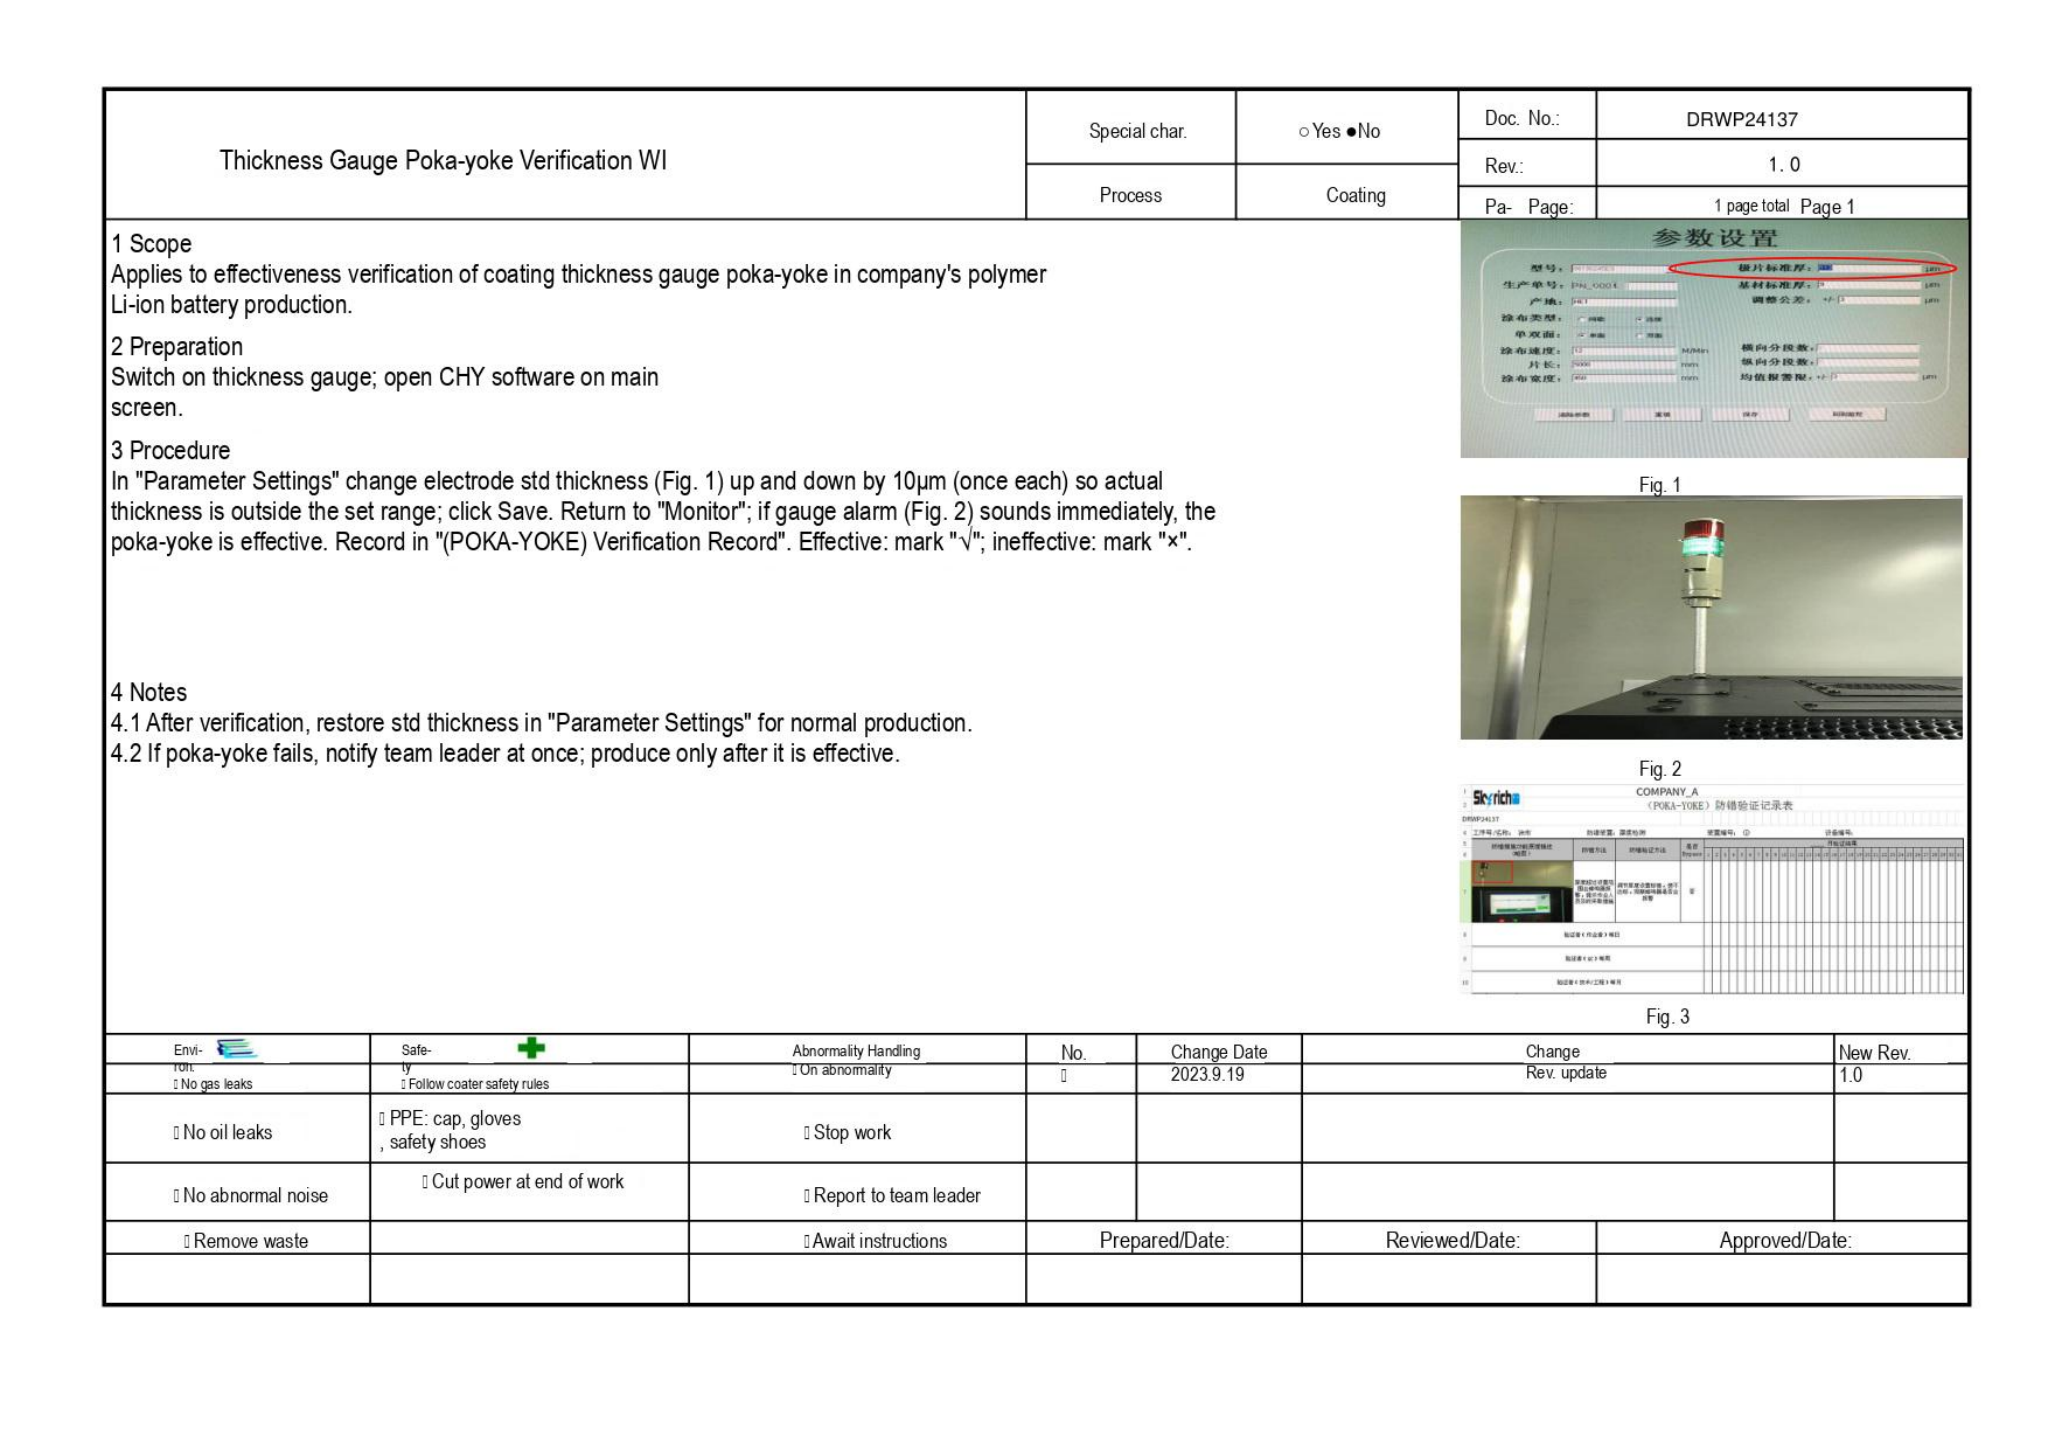# Thickness Gauge Poka-yoke Verification WI

| Thickness Gauge Poka-yoke Verification WI | Special char. | ○Yes ●No | Doc. No.: | DRWP24137 |
|---|---|---|---|---|
| | Process | Coating | Rev.: | 1. 0 |
| | | | Pa- Page: | 1 page total Page 1 |

1 Scope
Applies to effectiveness verification of coating thickness gauge poka-yoke in company's polymer Li-ion battery production.

2 Preparation
Switch on thickness gauge; open CHY software on main screen.

3 Procedure
In "Parameter Settings" change electrode std thickness (Fig. 1) up and down by 10μm (once each) so actual thickness is outside the set range; click Save. Return to "Monitor"; if gauge alarm (Fig. 2) sounds immediately, the poka-yoke is effective. Record in "(POKA-YOKE) Verification Record". Effective: mark "√"; ineffective: mark "×".

4 Notes
4.1 After verification, restore std thickness in "Parameter Settings" for normal production.
4.2 If poka-yoke fails, notify team leader at once; produce only after it is effective.

参数设置
型号: 生产单号: 产线: 涂布类型: 单双面: 涂布速度: M/Min 片长: mm 涂布宽度: mm
极片标准厚: μm 基材标准厚: μm 调整公差: +/- μm 横向分段数: 纵向分段数: 均值报警限: +/- μm

Fig. 1

Fig. 2

Skyrich
COMPANY_A
(POKA-YOKE) 防错验证记录表
DRWP24137

Fig. 3

| Envi-ron. | Safe-ty | Abnormality Handling | No. | Change Date | Change | New Rev. |
|---|---|---|---|---|---|---|
| No gas leaks | Follow coater safety rules | On abnormality | | 2023.9.19 | Rev. update | 1.0 |
| No oil leaks | PPE: cap, gloves, safety shoes | Stop work | | | | |
| No abnormal noise | Cut power at end of work | Report to team leader | | | | |
| Remove waste | | Await instructions | Prepared/Date: | | Reviewed/Date: | Approved/Date: |
| | | | | | | |